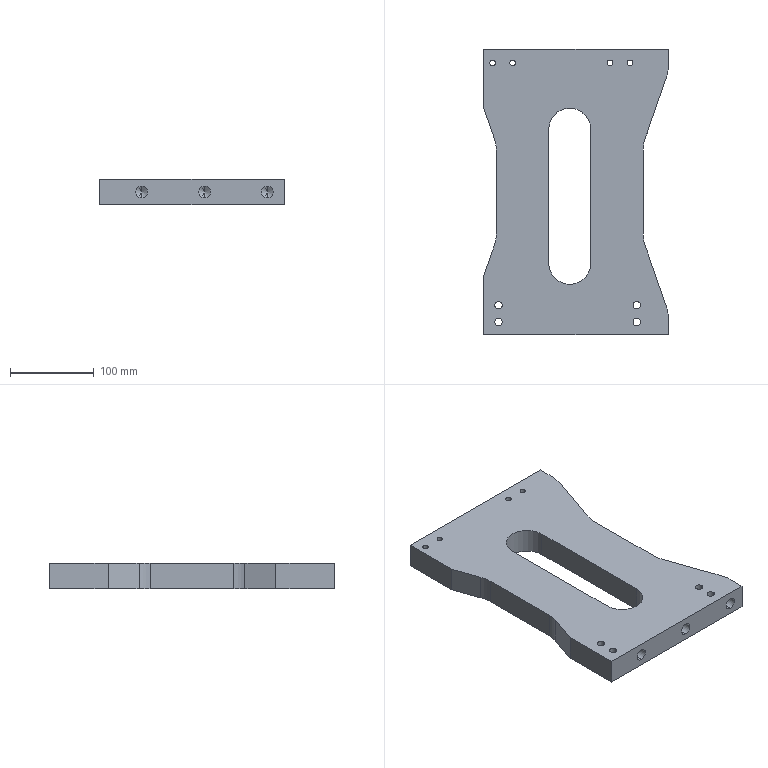Part | SolidWorks | features HoleWzd 4, Cut 1, Extrusion 1 | 1 solid | 64 faces | box 220 x 340 x 30 mm | volume 1630627 mm3 | cylinder 36 | plane 16 | cone 12 | commonest cylinder face diameters 14 x12 6.8 x8 9 x8 80 x6 50 x2